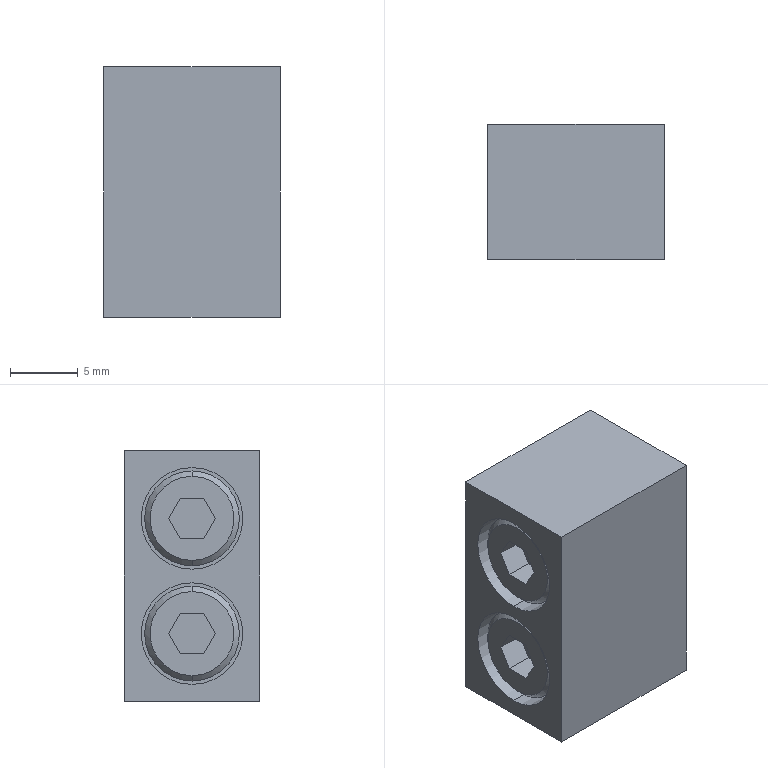Part | SolidWorks | features BaseBody 1 | 1 solid | 36 faces | box 13 x 10 x 18.5 mm | volume 2290 mm3 | plane 24 | cylinder 8 | cone 4 | commonest cylinder face diameters 7 x4 7.5 x4
STEP:
#1=CARTESIAN_POINT('',(-12.6,0.,7.35));
#2=VERTEX_POINT('',#1);
#3=CARTESIAN_POINT('',(-12.6,0.,1.15));
#4=VERTEX_POINT('',#3);
#5=CARTESIAN_POINT('',(-12.6,0.,4.25));
#6=DIRECTION('',(-1.,0.,0.));
#7=DIRECTION('',(0.,0.,1.));
#8=AXIS2_PLACEMENT_3D('',#5,#6,#7);
#9=CIRCLE('',#8,3.1);
#10=EDGE_CURVE('',#2,#4,#9,.T.);
#11=ORIENTED_EDGE('',*,*,#10,.F.);
#12=CARTESIAN_POINT('',(-12.2,0.,7.75));
#13=VERTEX_POINT('',#12);
#14=CARTESIAN_POINT('',(-12.2,0.,7.75));
#15=DIRECTION('',(0.7071,0.,0.7071));
#16=VECTOR('',#15,1000.);
#17=LINE('',#14,#16);
#18=EDGE_CURVE('',#2,#13,#17,.T.);
#19=ORIENTED_EDGE('',*,*,#18,.T.);
#20=CARTESIAN_POINT('',(-12.2,0.,0.75));
#21=VERTEX_POINT('',#20);
#22=CARTESIAN_POINT('',(-12.2,0.,4.25));
#23=DIRECTION('',(-1.,0.,0.));
#24=DIRECTION('',(0.,0.,1.));
#25=AXIS2_PLACEMENT_3D('',#22,#23,#24);
#26=CIRCLE('',#25,3.5);
#27=EDGE_CURVE('',#13,#21,#26,.T.);
#28=ORIENTED_EDGE('',*,*,#27,.T.);
#29=CARTESIAN_POINT('',(-12.2,0.,0.75));
#30=DIRECTION('',(0.7071,0.,-0.7071));
#31=VECTOR('',#30,1000.);
#32=LINE('',#29,#31);
#33=EDGE_CURVE('',#4,#21,#32,.T.);
#34=ORIENTED_EDGE('',*,*,#33,.F.);
#35=EDGE_LOOP('',(#11,#19,#28,#34));
#36=FACE_OUTER_BOUND('',#35,.T.);
#37=CARTESIAN_POINT('',(-12.2,0.,4.25));
#38=DIRECTION('',(1.,0.,0.));
#39=DIRECTION('',(0.,0.,-1.));
#40=AXIS2_PLACEMENT_3D('',#37,#38,#39);
#41=CONICAL_SURFACE('',#40,3.5,0.7854);
#42=ADVANCED_FACE('',(#36),#41,.T.);
#43=CARTESIAN_POINT('',(-8.6,0.,7.75));
#44=VERTEX_POINT('',#43);
#45=CARTESIAN_POINT('',(-8.6,0.,0.75));
#46=VERTEX_POINT('',#45);
#47=CARTESIAN_POINT('',(-8.6,0.,4.25));
#48=DIRECTION('',(-1.,0.,0.));
#49=DIRECTION('',(0.,0.,-1.));
#50=AXIS2_PLACEMENT_3D('',#47,#48,#49);
#51=CIRCLE('',#50,3.5);
#52=EDGE_CURVE('',#44,#46,#51,.T.);
#53=ORIENTED_EDGE('',*,*,#52,.T.);
#54=CARTESIAN_POINT('',(-12.6,0.,0.75));
#55=DIRECTION('',(-1.,0.,0.));
#56=VECTOR('',#55,1000.);
#57=LINE('',#54,#56);
#58=EDGE_CURVE('',#46,#21,#57,.T.);
#59=ORIENTED_EDGE('',*,*,#58,.T.);
#60=ORIENTED_EDGE('',*,*,#27,.F.);
#61=CARTESIAN_POINT('',(-12.6,0.,7.75));
#62=DIRECTION('',(-1.,0.,0.));
#63=VECTOR('',#62,1000.);
#64=LINE('',#61,#63);
#65=EDGE_CURVE('',#44,#13,#64,.T.);
#66=ORIENTED_EDGE('',*,*,#65,.F.);
#67=EDGE_LOOP('',(#53,#59,#60,#66));
#68=FACE_OUTER_BOUND('',#67,.T.);
#69=CARTESIAN_POINT('',(-12.6,0.,4.25));
#70=DIRECTION('',(-1.,0.,0.));
#71=DIRECTION('',(0.,0.,1.));
#72=AXIS2_PLACEMENT_3D('',#69,#70,#71);
#73=CYLINDRICAL_SURFACE('',#72,3.5);
#74=ADVANCED_FACE('',(#68),#73,.T.);
#75=CARTESIAN_POINT('',(-8.6,0.,8.));
#76=VERTEX_POINT('',#75);
#77=CARTESIAN_POINT('',(-8.6,0.,0.5));
#78=VERTEX_POINT('',#77);
#79=CARTESIAN_POINT('',(-8.6,0.,4.25));
#80=DIRECTION('',(1.,0.,0.));
#81=DIRECTION('',(0.,0.,-1.));
#82=AXIS2_PLACEMENT_3D('',#79,#80,#81);
#83=CIRCLE('',#82,3.75);
#84=EDGE_CURVE('',#76,#78,#83,.T.);
#85=ORIENTED_EDGE('',*,*,#84,.T.);
#86=CARTESIAN_POINT('',(-13.,0.,0.5));
#87=VERTEX_POINT('',#86);
#88=CARTESIAN_POINT('',(-8.6,0.,0.5));
#89=DIRECTION('',(-1.,0.,0.));
#90=VECTOR('',#89,1000.);
#91=LINE('',#88,#90);
#92=EDGE_CURVE('',#78,#87,#91,.T.);
#93=ORIENTED_EDGE('',*,*,#92,.T.);
#94=CARTESIAN_POINT('',(-13.,0.,8.));
#95=VERTEX_POINT('',#94);
#96=CARTESIAN_POINT('',(-13.,0.,4.25));
#97=DIRECTION('',(1.,0.,0.));
#98=DIRECTION('',(0.,0.,-1.));
#99=AXIS2_PLACEMENT_3D('',#96,#97,#98);
#100=CIRCLE('',#99,3.75);
#101=EDGE_CURVE('',#95,#87,#100,.T.);
#102=ORIENTED_EDGE('',*,*,#101,.F.);
#103=CARTESIAN_POINT('',(-8.6,0.,8.));
#104=DIRECTION('',(-1.,0.,0.));
#105=VECTOR('',#104,1000.);
#106=LINE('',#103,#105);
#107=EDGE_CURVE('',#76,#95,#106,.T.);
#108=ORIENTED_EDGE('',*,*,#107,.F.);
#109=EDGE_LOOP('',(#85,#93,#102,#108));
#110=FACE_OUTER_BOUND('',#109,.T.);
#111=CARTESIAN_POINT('',(-8.6,0.,4.25));
#112=DIRECTION('',(-1.,0.,0.));
#113=DIRECTION('',(0.,0.,1.));
#114=AXIS2_PLACEMENT_3D('',#111,#112,#113);
#115=CYLINDRICAL_SURFACE('',#114,3.75);
#116=ADVANCED_FACE('',(#110),#115,.F.);
#117=CARTESIAN_POINT('',(-8.6,0.,-0.5));
#118=VERTEX_POINT('',#117);
#119=CARTESIAN_POINT('',(-8.6,0.,-8.));
#120=VERTEX_POINT('',#119);
#121=CARTESIAN_POINT('',(-8.6,0.,-4.25));
#122=DIRECTION('',(1.,0.,0.));
#123=DIRECTION('',(0.,0.,-1.));
#124=AXIS2_PLACEMENT_3D('',#121,#122,#123);
#125=CIRCLE('',#124,3.75);
#126=EDGE_CURVE('',#118,#120,#125,.T.);
#127=ORIENTED_EDGE('',*,*,#126,.T.);
#128=CARTESIAN_POINT('',(-13.,0.,-8.));
#129=VERTEX_POINT('',#128);
#130=CARTESIAN_POINT('',(-8.6,0.,-8.));
#131=DIRECTION('',(-1.,0.,0.));
#132=VECTOR('',#131,1000.);
#133=LINE('',#130,#132);
#134=EDGE_CURVE('',#120,#129,#133,.T.);
#135=ORIENTED_EDGE('',*,*,#134,.T.);
#136=CARTESIAN_POINT('',(-13.,0.,-0.5));
#137=VERTEX_POINT('',#136);
#138=CARTESIAN_POINT('',(-13.,0.,-4.25));
#139=DIRECTION('',(1.,0.,0.));
#140=DIRECTION('',(0.,0.,-1.));
#141=AXIS2_PLACEMENT_3D('',#138,#139,#140);
#142=CIRCLE('',#141,3.75);
#143=EDGE_CURVE('',#137,#129,#142,.T.);
#144=ORIENTED_EDGE('',*,*,#143,.F.);
#145=CARTESIAN_POINT('',(-8.6,0.,-0.5));
#146=DIRECTION('',(-1.,0.,0.));
#147=VECTOR('',#146,1000.);
#148=LINE('',#145,#147);
#149=EDGE_CURVE('',#118,#137,#148,.T.);
#150=ORIENTED_EDGE('',*,*,#149,.F.);
#151=EDGE_LOOP('',(#127,#135,#144,#150));
#152=FACE_OUTER_BOUND('',#151,.T.);
#153=CARTESIAN_POINT('',(-8.6,0.,-4.25));
#154=DIRECTION('',(-1.,0.,0.));
#155=DIRECTION('',(0.,0.,1.));
#156=AXIS2_PLACEMENT_3D('',#153,#154,#155);
#157=CYLINDRICAL_SURFACE('',#156,3.75);
#158=ADVANCED_FACE('',(#152),#157,.F.);
#159=CARTESIAN_POINT('',(-8.6,0.,-0.75));
#160=VERTEX_POINT('',#159);
#161=CARTESIAN_POINT('',(-8.6,0.,-7.75));
#162=VERTEX_POINT('',#161);
#163=CARTESIAN_POINT('',(-8.6,0.,-4.25));
#164=DIRECTION('',(-1.,0.,0.));
#165=DIRECTION('',(0.,0.,-1.));
#166=AXIS2_PLACEMENT_3D('',#163,#164,#165);
#167=CIRCLE('',#166,3.5);
#168=EDGE_CURVE('',#160,#162,#167,.T.);
#169=ORIENTED_EDGE('',*,*,#168,.T.);
#170=CARTESIAN_POINT('',(-12.2,0.,-7.75));
#171=VERTEX_POINT('',#170);
#172=CARTESIAN_POINT('',(-12.6,0.,-7.75));
#173=DIRECTION('',(-1.,0.,0.));
#174=VECTOR('',#173,1000.);
#175=LINE('',#172,#174);
#176=EDGE_CURVE('',#162,#171,#175,.T.);
#177=ORIENTED_EDGE('',*,*,#176,.T.);
#178=CARTESIAN_POINT('',(-12.2,0.,-0.75));
#179=VERTEX_POINT('',#178);
#180=CARTESIAN_POINT('',(-12.2,0.,-4.25));
#181=DIRECTION('',(-1.,0.,0.));
#182=DIRECTION('',(0.,0.,1.));
#183=AXIS2_PLACEMENT_3D('',#180,#181,#182);
#184=CIRCLE('',#183,3.5);
#185=EDGE_CURVE('',#179,#171,#184,.T.);
#186=ORIENTED_EDGE('',*,*,#185,.F.);
#187=CARTESIAN_POINT('',(-12.6,0.,-0.75));
#188=DIRECTION('',(-1.,0.,0.));
#189=VECTOR('',#188,1000.);
#190=LINE('',#187,#189);
#191=EDGE_CURVE('',#160,#179,#190,.T.);
#192=ORIENTED_EDGE('',*,*,#191,.F.);
#193=EDGE_LOOP('',(#169,#177,#186,#192));
#194=FACE_OUTER_BOUND('',#193,.T.);
#195=CARTESIAN_POINT('',(-12.6,0.,-4.25));
#196=DIRECTION('',(-1.,0.,0.));
#197=DIRECTION('',(0.,0.,1.));
#198=AXIS2_PLACEMENT_3D('',#195,#196,#197);
#199=CYLINDRICAL_SURFACE('',#198,3.5);
#200=ADVANCED_FACE('',(#194),#199,.T.);
#201=CARTESIAN_POINT('',(-12.6,0.,-1.15));
#202=VERTEX_POINT('',#201);
#203=CARTESIAN_POINT('',(-12.6,0.,-7.35));
#204=VERTEX_POINT('',#203);
#205=CARTESIAN_POINT('',(-12.6,0.,-4.25));
#206=DIRECTION('',(-1.,0.,0.));
#207=DIRECTION('',(0.,0.,1.));
#208=AXIS2_PLACEMENT_3D('',#205,#206,#207);
#209=CIRCLE('',#208,3.1);
#210=EDGE_CURVE('',#202,#204,#209,.T.);
#211=ORIENTED_EDGE('',*,*,#210,.F.);
#212=CARTESIAN_POINT('',(-12.2,0.,-0.75));
#213=DIRECTION('',(0.7071,0.,0.7071));
#214=VECTOR('',#213,1000.);
#215=LINE('',#212,#214);
#216=EDGE_CURVE('',#202,#179,#215,.T.);
#217=ORIENTED_EDGE('',*,*,#216,.T.);
#218=ORIENTED_EDGE('',*,*,#185,.T.);
#219=CARTESIAN_POINT('',(-12.2,0.,-7.75));
#220=DIRECTION('',(0.7071,0.,-0.7071));
#221=VECTOR('',#220,1000.);
#222=LINE('',#219,#221);
#223=EDGE_CURVE('',#204,#171,#222,.T.);
#224=ORIENTED_EDGE('',*,*,#223,.F.);
#225=EDGE_LOOP('',(#211,#217,#218,#224));
#226=FACE_OUTER_BOUND('',#225,.T.);
#227=CARTESIAN_POINT('',(-12.2,0.,-4.25));
#228=DIRECTION('',(1.,0.,0.));
#229=DIRECTION('',(0.,0.,-1.));
#230=AXIS2_PLACEMENT_3D('',#227,#228,#229);
#231=CONICAL_SURFACE('',#230,3.5,0.7854);
#232=ADVANCED_FACE('',(#226),#231,.T.);
#233=CARTESIAN_POINT('',(-12.6,1.732,-4.25));
#234=VERTEX_POINT('',#233);
#235=CARTESIAN_POINT('',(-12.6,0.866,-2.75));
#236=VERTEX_POINT('',#235);
#237=CARTESIAN_POINT('',(-12.6,1.732,-4.25));
#238=DIRECTION('',(0.,-0.5,0.866));
#239=VECTOR('',#238,1000.);
#240=LINE('',#237,#239);
#241=EDGE_CURVE('',#234,#236,#240,.T.);
#242=ORIENTED_EDGE('',*,*,#241,.T.);
#243=CARTESIAN_POINT('',(-12.6,-0.866,-2.75));
#244=VERTEX_POINT('',#243);
#245=CARTESIAN_POINT('',(-12.6,-0.866,-2.75));
#246=DIRECTION('',(0.,1.,0.));
#247=VECTOR('',#246,1000.);
#248=LINE('',#245,#247);
#249=EDGE_CURVE('',#244,#236,#248,.T.);
#250=ORIENTED_EDGE('',*,*,#249,.F.);
#251=CARTESIAN_POINT('',(-12.6,-1.732,-4.25));
#252=VERTEX_POINT('',#251);
#253=CARTESIAN_POINT('',(-12.6,-0.866,-2.75));
#254=DIRECTION('',(0.,-0.5,-0.866));
#255=VECTOR('',#254,1000.);
#256=LINE('',#253,#255);
#257=EDGE_CURVE('',#244,#252,#256,.T.);
#258=ORIENTED_EDGE('',*,*,#257,.T.);
#259=CARTESIAN_POINT('',(-12.6,-0.866,-5.75));
#260=VERTEX_POINT('',#259);
#261=CARTESIAN_POINT('',(-12.6,-1.732,-4.25));
#262=DIRECTION('',(0.,0.5,-0.866));
#263=VECTOR('',#262,1000.);
#264=LINE('',#261,#263);
#265=EDGE_CURVE('',#252,#260,#264,.T.);
#266=ORIENTED_EDGE('',*,*,#265,.T.);
#267=CARTESIAN_POINT('',(-12.6,0.866,-5.75));
#268=VERTEX_POINT('',#267);
#269=CARTESIAN_POINT('',(-12.6,-0.866,-5.75));
#270=DIRECTION('',(0.,1.,0.));
#271=VECTOR('',#270,1000.);
#272=LINE('',#269,#271);
#273=EDGE_CURVE('',#260,#268,#272,.T.);
#274=ORIENTED_EDGE('',*,*,#273,.T.);
#275=CARTESIAN_POINT('',(-12.6,0.866,-5.75));
#276=DIRECTION('',(0.,0.5,0.866));
#277=VECTOR('',#276,1000.);
#278=LINE('',#275,#277);
#279=EDGE_CURVE('',#268,#234,#278,.T.);
#280=ORIENTED_EDGE('',*,*,#279,.T.);
#281=EDGE_LOOP('',(#242,#250,#258,#266,#274,#280));
#282=FACE_BOUND('',#281,.T.);
#283=CARTESIAN_POINT('',(-12.6,0.,-4.25));
#284=DIRECTION('',(-1.,0.,0.));
#285=DIRECTION('',(0.,0.,1.));
#286=AXIS2_PLACEMENT_3D('',#283,#284,#285);
#287=CIRCLE('',#286,3.1);
#288=EDGE_CURVE('',#204,#202,#287,.T.);
#289=ORIENTED_EDGE('',*,*,#288,.T.);
#290=ORIENTED_EDGE('',*,*,#210,.T.);
#291=EDGE_LOOP('',(#289,#290));
#292=FACE_OUTER_BOUND('',#291,.T.);
#293=CARTESIAN_POINT('',(-12.6,0.,-1.15));
#294=DIRECTION('',(1.,0.,0.));
#295=DIRECTION('',(0.,0.,-1.));
#296=AXIS2_PLACEMENT_3D('',#293,#294,#295);
#297=PLANE('',#296);
#298=ADVANCED_FACE('',(#282,#292),#297,.F.);
#299=ORIENTED_EDGE('',*,*,#241,.F.);
#300=CARTESIAN_POINT('',(-10.6,1.732,-4.25));
#301=VERTEX_POINT('',#300);
#302=CARTESIAN_POINT('',(-10.6,1.732,-4.25));
#303=DIRECTION('',(-1.,0.,0.));
#304=VECTOR('',#303,1000.);
#305=LINE('',#302,#304);
#306=EDGE_CURVE('',#301,#234,#305,.T.);
#307=ORIENTED_EDGE('',*,*,#306,.F.);
#308=CARTESIAN_POINT('',(-10.6,0.866,-2.75));
#309=VERTEX_POINT('',#308);
#310=CARTESIAN_POINT('',(-10.6,1.732,-4.25));
#311=DIRECTION('',(0.,-0.5,0.866));
#312=VECTOR('',#311,1000.);
#313=LINE('',#310,#312);
#314=EDGE_CURVE('',#301,#309,#313,.T.);
#315=ORIENTED_EDGE('',*,*,#314,.T.);
#316=CARTESIAN_POINT('',(-10.6,0.866,-2.75));
#317=DIRECTION('',(-1.,0.,0.));
#318=VECTOR('',#317,1000.);
#319=LINE('',#316,#318);
#320=EDGE_CURVE('',#309,#236,#319,.T.);
#321=ORIENTED_EDGE('',*,*,#320,.T.);
#322=EDGE_LOOP('',(#299,#307,#315,#321));
#323=FACE_OUTER_BOUND('',#322,.T.);
#324=CARTESIAN_POINT('',(-10.6,1.732,-4.25));
#325=DIRECTION('',(0.,-0.866,-0.5));
#326=DIRECTION('',(0.,0.5,-0.866));
#327=AXIS2_PLACEMENT_3D('',#324,#325,#326);
#328=PLANE('',#327);
#329=ADVANCED_FACE('',(#323),#328,.T.);
#330=ORIENTED_EDGE('',*,*,#249,.T.);
#331=ORIENTED_EDGE('',*,*,#320,.F.);
#332=CARTESIAN_POINT('',(-10.6,-0.866,-2.75));
#333=VERTEX_POINT('',#332);
#334=CARTESIAN_POINT('',(-10.6,0.866,-2.75));
#335=DIRECTION('',(0.,-1.,0.));
#336=VECTOR('',#335,1000.);
#337=LINE('',#334,#336);
#338=EDGE_CURVE('',#309,#333,#337,.T.);
#339=ORIENTED_EDGE('',*,*,#338,.T.);
#340=CARTESIAN_POINT('',(-10.6,-0.866,-2.75));
#341=DIRECTION('',(-1.,0.,0.));
#342=VECTOR('',#341,1000.);
#343=LINE('',#340,#342);
#344=EDGE_CURVE('',#333,#244,#343,.T.);
#345=ORIENTED_EDGE('',*,*,#344,.T.);
#346=EDGE_LOOP('',(#330,#331,#339,#345));
#347=FACE_OUTER_BOUND('',#346,.T.);
#348=CARTESIAN_POINT('',(-10.6,0.866,-2.75));
#349=DIRECTION('',(0.,0.,-1.));
#350=DIRECTION('',(-1.,0.,0.));
#351=AXIS2_PLACEMENT_3D('',#348,#349,#350);
#352=PLANE('',#351);
#353=ADVANCED_FACE('',(#347),#352,.T.);
#354=ORIENTED_EDGE('',*,*,#257,.F.);
#355=ORIENTED_EDGE('',*,*,#344,.F.);
#356=CARTESIAN_POINT('',(-10.6,-1.732,-4.25));
#357=VERTEX_POINT('',#356);
#358=CARTESIAN_POINT('',(-10.6,-0.866,-2.75));
#359=DIRECTION('',(0.,-0.5,-0.866));
#360=VECTOR('',#359,1000.);
#361=LINE('',#358,#360);
#362=EDGE_CURVE('',#333,#357,#361,.T.);
#363=ORIENTED_EDGE('',*,*,#362,.T.);
#364=CARTESIAN_POINT('',(-10.6,-1.732,-4.25));
#365=DIRECTION('',(-1.,0.,0.));
#366=VECTOR('',#365,1000.);
#367=LINE('',#364,#366);
#368=EDGE_CURVE('',#357,#252,#367,.T.);
#369=ORIENTED_EDGE('',*,*,#368,.T.);
#370=EDGE_LOOP('',(#354,#355,#363,#369));
#371=FACE_OUTER_BOUND('',#370,.T.);
#372=CARTESIAN_POINT('',(-10.6,-0.866,-2.75));
#373=DIRECTION('',(0.,0.866,-0.5));
#374=DIRECTION('',(0.,0.5,0.866));
#375=AXIS2_PLACEMENT_3D('',#372,#373,#374);
#376=PLANE('',#375);
#377=ADVANCED_FACE('',(#371),#376,.T.);
#378=ORIENTED_EDGE('',*,*,#265,.F.);
#379=ORIENTED_EDGE('',*,*,#368,.F.);
#380=CARTESIAN_POINT('',(-10.6,-0.866,-5.75));
#381=VERTEX_POINT('',#380);
#382=CARTESIAN_POINT('',(-10.6,-1.732,-4.25));
#383=DIRECTION('',(0.,0.5,-0.866));
#384=VECTOR('',#383,1000.);
#385=LINE('',#382,#384);
#386=EDGE_CURVE('',#357,#381,#385,.T.);
#387=ORIENTED_EDGE('',*,*,#386,.T.);
#388=CARTESIAN_POINT('',(-10.6,-0.866,-5.75));
#389=DIRECTION('',(-1.,0.,0.));
#390=VECTOR('',#389,1000.);
#391=LINE('',#388,#390);
#392=EDGE_CURVE('',#381,#260,#391,.T.);
#393=ORIENTED_EDGE('',*,*,#392,.T.);
#394=EDGE_LOOP('',(#378,#379,#387,#393));
#395=FACE_OUTER_BOUND('',#394,.T.);
#396=CARTESIAN_POINT('',(-10.6,-1.732,-4.25));
#397=DIRECTION('',(0.,0.866,0.5));
#398=DIRECTION('',(0.,-0.5,0.866));
#399=AXIS2_PLACEMENT_3D('',#396,#397,#398);
#400=PLANE('',#399);
#401=ADVANCED_FACE('',(#395),#400,.T.);
#402=ORIENTED_EDGE('',*,*,#273,.F.);
#403=ORIENTED_EDGE('',*,*,#392,.F.);
#404=CARTESIAN_POINT('',(-10.6,0.866,-5.75));
#405=VERTEX_POINT('',#404);
#406=CARTESIAN_POINT('',(-10.6,-0.866,-5.75));
#407=DIRECTION('',(0.,1.,0.));
#408=VECTOR('',#407,1000.);
#409=LINE('',#406,#408);
#410=EDGE_CURVE('',#381,#405,#409,.T.);
#411=ORIENTED_EDGE('',*,*,#410,.T.);
#412=CARTESIAN_POINT('',(-10.6,0.866,-5.75));
#413=DIRECTION('',(-1.,0.,0.));
#414=VECTOR('',#413,1000.);
#415=LINE('',#412,#414);
#416=EDGE_CURVE('',#405,#268,#415,.T.);
#417=ORIENTED_EDGE('',*,*,#416,.T.);
#418=EDGE_LOOP('',(#402,#403,#411,#417));
#419=FACE_OUTER_BOUND('',#418,.T.);
#420=CARTESIAN_POINT('',(-10.6,-0.866,-5.75));
#421=DIRECTION('',(0.,0.,1.));
#422=DIRECTION('',(1.,0.,0.));
#423=AXIS2_PLACEMENT_3D('',#420,#421,#422);
#424=PLANE('',#423);
#425=ADVANCED_FACE('',(#419),#424,.T.);
#426=ORIENTED_EDGE('',*,*,#279,.F.);
#427=ORIENTED_EDGE('',*,*,#416,.F.);
#428=CARTESIAN_POINT('',(-10.6,0.866,-5.75));
#429=DIRECTION('',(0.,0.5,0.866));
#430=VECTOR('',#429,1000.);
#431=LINE('',#428,#430);
#432=EDGE_CURVE('',#405,#301,#431,.T.);
#433=ORIENTED_EDGE('',*,*,#432,.T.);
#434=ORIENTED_EDGE('',*,*,#306,.T.);
#435=EDGE_LOOP('',(#426,#427,#433,#434));
#436=FACE_OUTER_BOUND('',#435,.T.);
#437=CARTESIAN_POINT('',(-10.6,0.866,-5.75));
#438=DIRECTION('',(0.,-0.866,0.5));
#439=DIRECTION('',(0.,-0.5,-0.866));
#440=AXIS2_PLACEMENT_3D('',#437,#438,#439);
#441=PLANE('',#440);
#442=ADVANCED_FACE('',(#436),#441,.T.);
#443=ORIENTED_EDGE('',*,*,#216,.F.);
#444=ORIENTED_EDGE('',*,*,#288,.F.);
#445=ORIENTED_EDGE('',*,*,#223,.T.);
#446=CARTESIAN_POINT('',(-12.2,0.,-4.25));
#447=DIRECTION('',(-1.,0.,0.));
#448=DIRECTION('',(0.,0.,1.));
#449=AXIS2_PLACEMENT_3D('',#446,#447,#448);
#450=CIRCLE('',#449,3.5);
#451=EDGE_CURVE('',#171,#179,#450,.T.);
#452=ORIENTED_EDGE('',*,*,#451,.T.);
#453=EDGE_LOOP('',(#443,#444,#445,#452));
#454=FACE_OUTER_BOUND('',#453,.T.);
#455=CARTESIAN_POINT('',(-12.2,0.,-4.25));
#456=DIRECTION('',(1.,0.,0.));
#457=DIRECTION('',(0.,0.,-1.));
#458=AXIS2_PLACEMENT_3D('',#455,#456,#457);
#459=CONICAL_SURFACE('',#458,3.5,0.7854);
#460=ADVANCED_FACE('',(#454),#459,.T.);
#461=ORIENTED_EDGE('',*,*,#338,.F.);
#462=ORIENTED_EDGE('',*,*,#314,.F.);
#463=ORIENTED_EDGE('',*,*,#432,.F.);
#464=ORIENTED_EDGE('',*,*,#410,.F.);
#465=ORIENTED_EDGE('',*,*,#386,.F.);
#466=ORIENTED_EDGE('',*,*,#362,.F.);
#467=EDGE_LOOP('',(#461,#462,#463,#464,#465,#466));
#468=FACE_OUTER_BOUND('',#467,.T.);
#469=CARTESIAN_POINT('',(-10.6,0.,-8.5));
#470=DIRECTION('',(1.,0.,0.));
#471=DIRECTION('',(0.,0.,-1.));
#472=AXIS2_PLACEMENT_3D('',#469,#470,#471);
#473=PLANE('',#472);
#474=ADVANCED_FACE('',(#468),#473,.F.);
#475=ORIENTED_EDGE('',*,*,#176,.F.);
#476=CARTESIAN_POINT('',(-8.6,0.,-4.25));
#477=DIRECTION('',(-1.,0.,0.));
#478=DIRECTION('',(0.,0.,-1.));
#479=AXIS2_PLACEMENT_3D('',#476,#477,#478);
#480=CIRCLE('',#479,3.5);
#481=EDGE_CURVE('',#162,#160,#480,.T.);
#482=ORIENTED_EDGE('',*,*,#481,.T.);
#483=ORIENTED_EDGE('',*,*,#191,.T.);
#484=ORIENTED_EDGE('',*,*,#451,.F.);
#485=EDGE_LOOP('',(#475,#482,#483,#484));
#486=FACE_OUTER_BOUND('',#485,.T.);
#487=CARTESIAN_POINT('',(-12.6,0.,-4.25));
#488=DIRECTION('',(-1.,0.,0.));
#489=DIRECTION('',(0.,0.,1.));
#490=AXIS2_PLACEMENT_3D('',#487,#488,#489);
#491=CYLINDRICAL_SURFACE('',#490,3.5);
#492=ADVANCED_FACE('',(#486),#491,.T.);
#493=ORIENTED_EDGE('',*,*,#168,.F.);
#494=ORIENTED_EDGE('',*,*,#481,.F.);
#495=EDGE_LOOP('',(#493,#494));
#496=FACE_BOUND('',#495,.T.);
#497=ORIENTED_EDGE('',*,*,#126,.F.);
#498=CARTESIAN_POINT('',(-8.6,0.,-4.25));
#499=DIRECTION('',(1.,0.,0.));
#500=DIRECTION('',(0.,0.,-1.));
#501=AXIS2_PLACEMENT_3D('',#498,#499,#500);
#502=CIRCLE('',#501,3.75);
#503=EDGE_CURVE('',#120,#118,#502,.T.);
#504=ORIENTED_EDGE('',*,*,#503,.F.);
#505=EDGE_LOOP('',(#497,#504));
#506=FACE_OUTER_BOUND('',#505,.T.);
#507=CARTESIAN_POINT('',(-8.6,0.,-4.25));
#508=DIRECTION('',(1.,0.,0.));
#509=DIRECTION('',(0.,0.,-1.));
#510=AXIS2_PLACEMENT_3D('',#507,#508,#509);
#511=PLANE('',#510);
#512=ADVANCED_FACE('',(#496,#506),#511,.F.);
#513=ORIENTED_EDGE('',*,*,#134,.F.);
#514=ORIENTED_EDGE('',*,*,#503,.T.);
#515=ORIENTED_EDGE('',*,*,#149,.T.);
#516=CARTESIAN_POINT('',(-13.,0.,-4.25));
#517=DIRECTION('',(1.,0.,0.));
#518=DIRECTION('',(0.,0.,-1.));
#519=AXIS2_PLACEMENT_3D('',#516,#517,#518);
#520=CIRCLE('',#519,3.75);
#521=EDGE_CURVE('',#129,#137,#520,.T.);
#522=ORIENTED_EDGE('',*,*,#521,.F.);
#523=EDGE_LOOP('',(#513,#514,#515,#522));
#524=FACE_OUTER_BOUND('',#523,.T.);
#525=CARTESIAN_POINT('',(-8.6,0.,-4.25));
#526=DIRECTION('',(-1.,0.,0.));
#527=DIRECTION('',(0.,0.,1.));
#528=AXIS2_PLACEMENT_3D('',#525,#526,#527);
#529=CYLINDRICAL_SURFACE('',#528,3.75);
#530=ADVANCED_FACE('',(#524),#529,.F.);
#531=ORIENTED_EDGE('',*,*,#143,.T.);
#532=ORIENTED_EDGE('',*,*,#521,.T.);
#533=EDGE_LOOP('',(#531,#532));
#534=FACE_BOUND('',#533,.T.);
#535=ORIENTED_EDGE('',*,*,#101,.T.);
#536=CARTESIAN_POINT('',(-13.,0.,4.25));
#537=DIRECTION('',(1.,0.,0.));
#538=DIRECTION('',(0.,0.,-1.));
#539=AXIS2_PLACEMENT_3D('',#536,#537,#538);
#540=CIRCLE('',#539,3.75);
#541=EDGE_CURVE('',#87,#95,#540,.T.);
#542=ORIENTED_EDGE('',*,*,#541,.T.);
#543=EDGE_LOOP('',(#535,#542));
#544=FACE_BOUND('',#543,.T.);
#545=CARTESIAN_POINT('',(-13.,-5.,-9.25));
#546=VERTEX_POINT('',#545);
#547=CARTESIAN_POINT('',(-13.,-5.,9.25));
#548=VERTEX_POINT('',#547);
#549=CARTESIAN_POINT('',(-13.,-5.,-9.25));
#550=DIRECTION('',(0.,0.,1.));
#551=VECTOR('',#550,1000.);
#552=LINE('',#549,#551);
#553=EDGE_CURVE('',#546,#548,#552,.T.);
#554=ORIENTED_EDGE('',*,*,#553,.T.);
#555=CARTESIAN_POINT('',(-13.,5.,9.25));
#556=VERTEX_POINT('',#555);
#557=CARTESIAN_POINT('',(-13.,5.,9.25));
#558=DIRECTION('',(0.,-1.,0.));
#559=VECTOR('',#558,1000.);
#560=LINE('',#557,#559);
#561=EDGE_CURVE('',#556,#548,#560,.T.);
#562=ORIENTED_EDGE('',*,*,#561,.F.);
#563=CARTESIAN_POINT('',(-13.,5.,-9.25));
#564=VERTEX_POINT('',#563);
#565=CARTESIAN_POINT('',(-13.,5.,-9.25));
#566=DIRECTION('',(0.,0.,1.));
#567=VECTOR('',#566,1000.);
#568=LINE('',#565,#567);
#569=EDGE_CURVE('',#564,#556,#568,.T.);
#570=ORIENTED_EDGE('',*,*,#569,.F.);
#571=CARTESIAN_POINT('',(-13.,5.,-9.25));
#572=DIRECTION('',(0.,-1.,0.));
#573=VECTOR('',#572,1000.);
#574=LINE('',#571,#573);
#575=EDGE_CURVE('',#564,#546,#574,.T.);
#576=ORIENTED_EDGE('',*,*,#575,.T.);
#577=EDGE_LOOP('',(#554,#562,#570,#576));
#578=FACE_OUTER_BOUND('',#577,.T.);
#579=CARTESIAN_POINT('',(-13.,5.,-9.25));
#580=DIRECTION('',(1.,0.,0.));
#581=DIRECTION('',(0.,0.,-1.));
#582=AXIS2_PLACEMENT_3D('',#579,#580,#581);
#583=PLANE('',#582);
#584=ADVANCED_FACE('',(#534,#544,#578),#583,.F.);
#585=ORIENTED_EDGE('',*,*,#92,.F.);
#586=CARTESIAN_POINT('',(-8.6,0.,4.25));
#587=DIRECTION('',(1.,0.,0.));
#588=DIRECTION('',(0.,0.,-1.));
#589=AXIS2_PLACEMENT_3D('',#586,#587,#588);
#590=CIRCLE('',#589,3.75);
#591=EDGE_CURVE('',#78,#76,#590,.T.);
#592=ORIENTED_EDGE('',*,*,#591,.T.);
#593=ORIENTED_EDGE('',*,*,#107,.T.);
#594=ORIENTED_EDGE('',*,*,#541,.F.);
#595=EDGE_LOOP('',(#585,#592,#593,#594));
#596=FACE_OUTER_BOUND('',#595,.T.);
#597=CARTESIAN_POINT('',(-8.6,0.,4.25));
#598=DIRECTION('',(-1.,0.,0.));
#599=DIRECTION('',(0.,0.,1.));
#600=AXIS2_PLACEMENT_3D('',#597,#598,#599);
#601=CYLINDRICAL_SURFACE('',#600,3.75);
#602=ADVANCED_FACE('',(#596),#601,.F.);
#603=CARTESIAN_POINT('',(0.,-5.,-9.25));
#604=VERTEX_POINT('',#603);
#605=CARTESIAN_POINT('',(0.,-5.,-9.25));
#606=DIRECTION('',(-1.,0.,0.));
#607=VECTOR('',#606,1000.);
#608=LINE('',#605,#607);
#609=EDGE_CURVE('',#604,#546,#608,.T.);
#610=ORIENTED_EDGE('',*,*,#609,.F.);
#611=CARTESIAN_POINT('',(0.,-5.,9.25));
#612=VERTEX_POINT('',#611);
#613=CARTESIAN_POINT('',(0.,-5.,9.25));
#614=DIRECTION('',(0.,0.,-1.));
#615=VECTOR('',#614,1000.);
#616=LINE('',#613,#615);
#617=EDGE_CURVE('',#612,#604,#616,.T.);
#618=ORIENTED_EDGE('',*,*,#617,.F.);
#619=CARTESIAN_POINT('',(-13.,-5.,9.25));
#620=DIRECTION('',(1.,0.,0.));
#621=VECTOR('',#620,1000.);
#622=LINE('',#619,#621);
#623=EDGE_CURVE('',#548,#612,#622,.T.);
#624=ORIENTED_EDGE('',*,*,#623,.F.);
#625=ORIENTED_EDGE('',*,*,#553,.F.);
#626=EDGE_LOOP('',(#610,#618,#624,#625));
#627=FACE_OUTER_BOUND('',#626,.T.);
#628=CARTESIAN_POINT('',(0.,-5.,0.));
#629=DIRECTION('',(0.,1.,0.));
#630=DIRECTION('',(0.,0.,1.));
#631=AXIS2_PLACEMENT_3D('',#628,#629,#630);
#632=PLANE('',#631);
#633=ADVANCED_FACE('',(#627),#632,.F.);
#634=ORIENTED_EDGE('',*,*,#623,.T.);
#635=CARTESIAN_POINT('',(0.,5.,9.25));
#636=VERTEX_POINT('',#635);
#637=CARTESIAN_POINT('',(0.,5.,9.25));
#638=DIRECTION('',(0.,-1.,0.));
#639=VECTOR('',#638,1000.);
#640=LINE('',#637,#639);
#641=EDGE_CURVE('',#636,#612,#640,.T.);
#642=ORIENTED_EDGE('',*,*,#641,.F.);
#643=CARTESIAN_POINT('',(-13.,5.,9.25));
#644=DIRECTION('',(1.,0.,0.));
#645=VECTOR('',#644,1000.);
#646=LINE('',#643,#645);
#647=EDGE_CURVE('',#556,#636,#646,.T.);
#648=ORIENTED_EDGE('',*,*,#647,.F.);
#649=ORIENTED_EDGE('',*,*,#561,.T.);
#650=EDGE_LOOP('',(#634,#642,#648,#649));
#651=FACE_OUTER_BOUND('',#650,.T.);
#652=CARTESIAN_POINT('',(-13.,5.,9.25));
#653=DIRECTION('',(0.,0.,-1.));
#654=DIRECTION('',(-1.,0.,0.));
#655=AXIS2_PLACEMENT_3D('',#652,#653,#654);
#656=PLANE('',#655);
#657=ADVANCED_FACE('',(#651),#656,.F.);
#658=CARTESIAN_POINT('',(0.,5.,-9.25));
#659=VERTEX_POINT('',#658);
#660=CARTESIAN_POINT('',(0.,5.,-9.25));
#661=DIRECTION('',(-1.,0.,0.));
#662=VECTOR('',#661,1000.);
#663=LINE('',#660,#662);
#664=EDGE_CURVE('',#659,#564,#663,.T.);
#665=ORIENTED_EDGE('',*,*,#664,.T.);
#666=ORIENTED_EDGE('',*,*,#569,.T.);
#667=ORIENTED_EDGE('',*,*,#647,.T.);
#668=CARTESIAN_POINT('',(0.,5.,9.25));
#669=DIRECTION('',(0.,0.,-1.));
#670=VECTOR('',#669,1000.);
#671=LINE('',#668,#670);
#672=EDGE_CURVE('',#636,#659,#671,.T.);
#673=ORIENTED_EDGE('',*,*,#672,.T.);
#674=EDGE_LOOP('',(#665,#666,#667,#673));
#675=FACE_OUTER_BOUND('',#674,.T.);
#676=CARTESIAN_POINT('',(0.,5.,0.));
#677=DIRECTION('',(0.,1.,0.));
#678=DIRECTION('',(0.,0.,1.));
#679=AXIS2_PLACEMENT_3D('',#676,#677,#678);
#680=PLANE('',#679);
#681=ADVANCED_FACE('',(#675),#680,.T.);
#682=ORIENTED_EDGE('',*,*,#609,.T.);
#683=ORIENTED_EDGE('',*,*,#575,.F.);
#684=ORIENTED_EDGE('',*,*,#664,.F.);
#685=CARTESIAN_POINT('',(0.,5.,-9.25));
#686=DIRECTION('',(0.,-1.,0.));
#687=VECTOR('',#686,1000.);
#688=LINE('',#685,#687);
#689=EDGE_CURVE('',#659,#604,#688,.T.);
#690=ORIENTED_EDGE('',*,*,#689,.T.);
#691=EDGE_LOOP('',(#682,#683,#684,#690));
#692=FACE_OUTER_BOUND('',#691,.T.);
#693=CARTESIAN_POINT('',(0.,5.,-9.25));
#694=DIRECTION('',(0.,0.,1.));
#695=DIRECTION('',(1.,0.,0.));
#696=AXIS2_PLACEMENT_3D('',#693,#694,#695);
#697=PLANE('',#696);
#698=ADVANCED_FACE('',(#692),#697,.F.);
#699=ORIENTED_EDGE('',*,*,#52,.F.);
#700=CARTESIAN_POINT('',(-8.6,0.,4.25));
#701=DIRECTION('',(-1.,0.,0.));
#702=DIRECTION('',(0.,0.,-1.));
#703=AXIS2_PLACEMENT_3D('',#700,#701,#702);
#704=CIRCLE('',#703,3.5);
#705=EDGE_CURVE('',#46,#44,#704,.T.);
#706=ORIENTED_EDGE('',*,*,#705,.F.);
#707=EDGE_LOOP('',(#699,#706));
#708=FACE_BOUND('',#707,.T.);
#709=ORIENTED_EDGE('',*,*,#84,.F.);
#710=ORIENTED_EDGE('',*,*,#591,.F.);
#711=EDGE_LOOP('',(#709,#710));
#712=FACE_OUTER_BOUND('',#711,.T.);
#713=CARTESIAN_POINT('',(-8.6,0.,4.25));
#714=DIRECTION('',(1.,0.,0.));
#715=DIRECTION('',(0.,0.,-1.));
#716=AXIS2_PLACEMENT_3D('',#713,#714,#715);
#717=PLANE('',#716);
#718=ADVANCED_FACE('',(#708,#712),#717,.F.);
#719=ORIENTED_EDGE('',*,*,#617,.T.);
#720=ORIENTED_EDGE('',*,*,#689,.F.);
#721=ORIENTED_EDGE('',*,*,#672,.F.);
#722=ORIENTED_EDGE('',*,*,#641,.T.);
#723=EDGE_LOOP('',(#719,#720,#721,#722));
#724=FACE_OUTER_BOUND('',#723,.T.);
#725=CARTESIAN_POINT('',(0.,5.,9.25));
#726=DIRECTION('',(-1.,0.,0.));
#727=DIRECTION('',(0.,0.,1.));
#728=AXIS2_PLACEMENT_3D('',#725,#726,#727);
#729=PLANE('',#728);
#730=ADVANCED_FACE('',(#724),#729,.F.);
#731=ORIENTED_EDGE('',*,*,#58,.F.);
#732=ORIENTED_EDGE('',*,*,#705,.T.);
#733=ORIENTED_EDGE('',*,*,#65,.T.);
#734=CARTESIAN_POINT('',(-12.2,0.,4.25));
#735=DIRECTION('',(-1.,0.,0.));
#736=DIRECTION('',(0.,0.,1.));
#737=AXIS2_PLACEMENT_3D('',#734,#735,#736);
#738=CIRCLE('',#737,3.5);
#739=EDGE_CURVE('',#21,#13,#738,.T.);
#740=ORIENTED_EDGE('',*,*,#739,.F.);
#741=EDGE_LOOP('',(#731,#732,#733,#740));
#742=FACE_OUTER_BOUND('',#741,.T.);
#743=CARTESIAN_POINT('',(-12.6,0.,4.25));
#744=DIRECTION('',(-1.,0.,0.));
#745=DIRECTION('',(0.,0.,1.));
#746=AXIS2_PLACEMENT_3D('',#743,#744,#745);
#747=CYLINDRICAL_SURFACE('',#746,3.5);
#748=ADVANCED_FACE('',(#742),#747,.T.);
#749=ORIENTED_EDGE('',*,*,#18,.F.);
#750=CARTESIAN_POINT('',(-12.6,0.,4.25));
#751=DIRECTION('',(-1.,0.,0.));
#752=DIRECTION('',(0.,0.,1.));
#753=AXIS2_PLACEMENT_3D('',#750,#751,#752);
#754=CIRCLE('',#753,3.1);
#755=EDGE_CURVE('',#4,#2,#754,.T.);
#756=ORIENTED_EDGE('',*,*,#755,.F.);
#757=ORIENTED_EDGE('',*,*,#33,.T.);
#758=ORIENTED_EDGE('',*,*,#739,.T.);
#759=EDGE_LOOP('',(#749,#756,#757,#758));
#760=FACE_OUTER_BOUND('',#759,.T.);
#761=CARTESIAN_POINT('',(-12.2,0.,4.25));
#762=DIRECTION('',(1.,0.,0.));
#763=DIRECTION('',(0.,0.,-1.));
#764=AXIS2_PLACEMENT_3D('',#761,#762,#763);
#765=CONICAL_SURFACE('',#764,3.5,0.7854);
#766=ADVANCED_FACE('',(#760),#765,.T.);
#767=CARTESIAN_POINT('',(-12.6,1.732,4.25));
#768=VERTEX_POINT('',#767);
#769=CARTESIAN_POINT('',(-12.6,0.866,5.75));
#770=VERTEX_POINT('',#769);
#771=CARTESIAN_POINT('',(-12.6,1.732,4.25));
#772=DIRECTION('',(0.,-0.5,0.866));
#773=VECTOR('',#772,1000.);
#774=LINE('',#771,#773);
#775=EDGE_CURVE('',#768,#770,#774,.T.);
#776=ORIENTED_EDGE('',*,*,#775,.T.);
#777=CARTESIAN_POINT('',(-12.6,-0.866,5.75));
#778=VERTEX_POINT('',#777);
#779=CARTESIAN_POINT('',(-12.6,-0.866,5.75));
#780=DIRECTION('',(0.,1.,0.));
#781=VECTOR('',#780,1000.);
#782=LINE('',#779,#781);
#783=EDGE_CURVE('',#778,#770,#782,.T.);
#784=ORIENTED_EDGE('',*,*,#783,.F.);
#785=CARTESIAN_POINT('',(-12.6,-1.732,4.25));
#786=VERTEX_POINT('',#785);
#787=CARTESIAN_POINT('',(-12.6,-0.866,5.75));
#788=DIRECTION('',(0.,-0.5,-0.866));
#789=VECTOR('',#788,1000.);
#790=LINE('',#787,#789);
#791=EDGE_CURVE('',#778,#786,#790,.T.);
#792=ORIENTED_EDGE('',*,*,#791,.T.);
#793=CARTESIAN_POINT('',(-12.6,-0.866,2.75));
#794=VERTEX_POINT('',#793);
#795=CARTESIAN_POINT('',(-12.6,-1.732,4.25));
#796=DIRECTION('',(0.,0.5,-0.866));
#797=VECTOR('',#796,1000.);
#798=LINE('',#795,#797);
#799=EDGE_CURVE('',#786,#794,#798,.T.);
#800=ORIENTED_EDGE('',*,*,#799,.T.);
#801=CARTESIAN_POINT('',(-12.6,0.866,2.75));
#802=VERTEX_POINT('',#801);
#803=CARTESIAN_POINT('',(-12.6,-0.866,2.75));
#804=DIRECTION('',(0.,1.,0.));
#805=VECTOR('',#804,1000.);
#806=LINE('',#803,#805);
#807=EDGE_CURVE('',#794,#802,#806,.T.);
#808=ORIENTED_EDGE('',*,*,#807,.T.);
#809=CARTESIAN_POINT('',(-12.6,0.866,2.75));
#810=DIRECTION('',(0.,0.5,0.866));
#811=VECTOR('',#810,1000.);
#812=LINE('',#809,#811);
#813=EDGE_CURVE('',#802,#768,#812,.T.);
#814=ORIENTED_EDGE('',*,*,#813,.T.);
#815=EDGE_LOOP('',(#776,#784,#792,#800,#808,#814));
#816=FACE_BOUND('',#815,.T.);
#817=ORIENTED_EDGE('',*,*,#755,.T.);
#818=ORIENTED_EDGE('',*,*,#10,.T.);
#819=EDGE_LOOP('',(#817,#818));
#820=FACE_OUTER_BOUND('',#819,.T.);
#821=CARTESIAN_POINT('',(-12.6,0.,7.35));
#822=DIRECTION('',(1.,0.,0.));
#823=DIRECTION('',(0.,0.,-1.));
#824=AXIS2_PLACEMENT_3D('',#821,#822,#823);
#825=PLANE('',#824);
#826=ADVANCED_FACE('',(#816,#820),#825,.F.);
#827=ORIENTED_EDGE('',*,*,#775,.F.);
#828=CARTESIAN_POINT('',(-10.6,1.732,4.25));
#829=VERTEX_POINT('',#828);
#830=CARTESIAN_POINT('',(-10.6,1.732,4.25));
#831=DIRECTION('',(-1.,0.,0.));
#832=VECTOR('',#831,1000.);
#833=LINE('',#830,#832);
#834=EDGE_CURVE('',#829,#768,#833,.T.);
#835=ORIENTED_EDGE('',*,*,#834,.F.);
#836=CARTESIAN_POINT('',(-10.6,0.866,5.75));
#837=VERTEX_POINT('',#836);
#838=CARTESIAN_POINT('',(-10.6,1.732,4.25));
#839=DIRECTION('',(0.,-0.5,0.866));
#840=VECTOR('',#839,1000.);
#841=LINE('',#838,#840);
#842=EDGE_CURVE('',#829,#837,#841,.T.);
#843=ORIENTED_EDGE('',*,*,#842,.T.);
#844=CARTESIAN_POINT('',(-10.6,0.866,5.75));
#845=DIRECTION('',(-1.,0.,0.));
#846=VECTOR('',#845,1000.);
#847=LINE('',#844,#846);
#848=EDGE_CURVE('',#837,#770,#847,.T.);
#849=ORIENTED_EDGE('',*,*,#848,.T.);
#850=EDGE_LOOP('',(#827,#835,#843,#849));
#851=FACE_OUTER_BOUND('',#850,.T.);
#852=CARTESIAN_POINT('',(-10.6,1.732,4.25));
#853=DIRECTION('',(0.,-0.866,-0.5));
#854=DIRECTION('',(0.,0.5,-0.866));
#855=AXIS2_PLACEMENT_3D('',#852,#853,#854);
#856=PLANE('',#855);
#857=ADVANCED_FACE('',(#851),#856,.T.);
#858=ORIENTED_EDGE('',*,*,#783,.T.);
#859=ORIENTED_EDGE('',*,*,#848,.F.);
#860=CARTESIAN_POINT('',(-10.6,-0.866,5.75));
#861=VERTEX_POINT('',#860);
#862=CARTESIAN_POINT('',(-10.6,0.866,5.75));
#863=DIRECTION('',(0.,-1.,0.));
#864=VECTOR('',#863,1000.);
#865=LINE('',#862,#864);
#866=EDGE_CURVE('',#837,#861,#865,.T.);
#867=ORIENTED_EDGE('',*,*,#866,.T.);
#868=CARTESIAN_POINT('',(-10.6,-0.866,5.75));
#869=DIRECTION('',(-1.,0.,0.));
#870=VECTOR('',#869,1000.);
#871=LINE('',#868,#870);
#872=EDGE_CURVE('',#861,#778,#871,.T.);
#873=ORIENTED_EDGE('',*,*,#872,.T.);
#874=EDGE_LOOP('',(#858,#859,#867,#873));
#875=FACE_OUTER_BOUND('',#874,.T.);
#876=CARTESIAN_POINT('',(-10.6,0.866,5.75));
#877=DIRECTION('',(0.,0.,-1.));
#878=DIRECTION('',(-1.,0.,0.));
#879=AXIS2_PLACEMENT_3D('',#876,#877,#878);
#880=PLANE('',#879);
#881=ADVANCED_FACE('',(#875),#880,.T.);
#882=ORIENTED_EDGE('',*,*,#791,.F.);
#883=ORIENTED_EDGE('',*,*,#872,.F.);
#884=CARTESIAN_POINT('',(-10.6,-1.732,4.25));
#885=VERTEX_POINT('',#884);
#886=CARTESIAN_POINT('',(-10.6,-0.866,5.75));
#887=DIRECTION('',(0.,-0.5,-0.866));
#888=VECTOR('',#887,1000.);
#889=LINE('',#886,#888);
#890=EDGE_CURVE('',#861,#885,#889,.T.);
#891=ORIENTED_EDGE('',*,*,#890,.T.);
#892=CARTESIAN_POINT('',(-10.6,-1.732,4.25));
#893=DIRECTION('',(-1.,0.,0.));
#894=VECTOR('',#893,1000.);
#895=LINE('',#892,#894);
#896=EDGE_CURVE('',#885,#786,#895,.T.);
#897=ORIENTED_EDGE('',*,*,#896,.T.);
#898=EDGE_LOOP('',(#882,#883,#891,#897));
#899=FACE_OUTER_BOUND('',#898,.T.);
#900=CARTESIAN_POINT('',(-10.6,-0.866,5.75));
#901=DIRECTION('',(0.,0.866,-0.5));
#902=DIRECTION('',(0.,0.5,0.866));
#903=AXIS2_PLACEMENT_3D('',#900,#901,#902);
#904=PLANE('',#903);
#905=ADVANCED_FACE('',(#899),#904,.T.);
#906=ORIENTED_EDGE('',*,*,#799,.F.);
#907=ORIENTED_EDGE('',*,*,#896,.F.);
#908=CARTESIAN_POINT('',(-10.6,-0.866,2.75));
#909=VERTEX_POINT('',#908);
#910=CARTESIAN_POINT('',(-10.6,-1.732,4.25));
#911=DIRECTION('',(0.,0.5,-0.866));
#912=VECTOR('',#911,1000.);
#913=LINE('',#910,#912);
#914=EDGE_CURVE('',#885,#909,#913,.T.);
#915=ORIENTED_EDGE('',*,*,#914,.T.);
#916=CARTESIAN_POINT('',(-10.6,-0.866,2.75));
#917=DIRECTION('',(-1.,0.,0.));
#918=VECTOR('',#917,1000.);
#919=LINE('',#916,#918);
#920=EDGE_CURVE('',#909,#794,#919,.T.);
#921=ORIENTED_EDGE('',*,*,#920,.T.);
#922=EDGE_LOOP('',(#906,#907,#915,#921));
#923=FACE_OUTER_BOUND('',#922,.T.);
#924=CARTESIAN_POINT('',(-10.6,-1.732,4.25));
#925=DIRECTION('',(0.,0.866,0.5));
#926=DIRECTION('',(0.,-0.5,0.866));
#927=AXIS2_PLACEMENT_3D('',#924,#925,#926);
#928=PLANE('',#927);
#929=ADVANCED_FACE('',(#923),#928,.T.);
#930=ORIENTED_EDGE('',*,*,#807,.F.);
#931=ORIENTED_EDGE('',*,*,#920,.F.);
#932=CARTESIAN_POINT('',(-10.6,0.866,2.75));
#933=VERTEX_POINT('',#932);
#934=CARTESIAN_POINT('',(-10.6,-0.866,2.75));
#935=DIRECTION('',(0.,1.,0.));
#936=VECTOR('',#935,1000.);
#937=LINE('',#934,#936);
#938=EDGE_CURVE('',#909,#933,#937,.T.);
#939=ORIENTED_EDGE('',*,*,#938,.T.);
#940=CARTESIAN_POINT('',(-10.6,0.866,2.75));
#941=DIRECTION('',(-1.,0.,0.));
#942=VECTOR('',#941,1000.);
#943=LINE('',#940,#942);
#944=EDGE_CURVE('',#933,#802,#943,.T.);
#945=ORIENTED_EDGE('',*,*,#944,.T.);
#946=EDGE_LOOP('',(#930,#931,#939,#945));
#947=FACE_OUTER_BOUND('',#946,.T.);
#948=CARTESIAN_POINT('',(-10.6,-0.866,2.75));
#949=DIRECTION('',(0.,0.,1.));
#950=DIRECTION('',(1.,0.,0.));
#951=AXIS2_PLACEMENT_3D('',#948,#949,#950);
#952=PLANE('',#951);
#953=ADVANCED_FACE('',(#947),#952,.T.);
#954=ORIENTED_EDGE('',*,*,#813,.F.);
#955=ORIENTED_EDGE('',*,*,#944,.F.);
#956=CARTESIAN_POINT('',(-10.6,0.866,2.75));
#957=DIRECTION('',(0.,0.5,0.866));
#958=VECTOR('',#957,1000.);
#959=LINE('',#956,#958);
#960=EDGE_CURVE('',#933,#829,#959,.T.);
#961=ORIENTED_EDGE('',*,*,#960,.T.);
#962=ORIENTED_EDGE('',*,*,#834,.T.);
#963=EDGE_LOOP('',(#954,#955,#961,#962));
#964=FACE_OUTER_BOUND('',#963,.T.);
#965=CARTESIAN_POINT('',(-10.6,0.866,2.75));
#966=DIRECTION('',(0.,-0.866,0.5));
#967=DIRECTION('',(0.,-0.5,-0.866));
#968=AXIS2_PLACEMENT_3D('',#965,#966,#967);
#969=PLANE('',#968);
#970=ADVANCED_FACE('',(#964),#969,.T.);
#971=ORIENTED_EDGE('',*,*,#866,.F.);
#972=ORIENTED_EDGE('',*,*,#842,.F.);
#973=ORIENTED_EDGE('',*,*,#960,.F.);
#974=ORIENTED_EDGE('',*,*,#938,.F.);
#975=ORIENTED_EDGE('',*,*,#914,.F.);
#976=ORIENTED_EDGE('',*,*,#890,.F.);
#977=EDGE_LOOP('',(#971,#972,#973,#974,#975,#976));
#978=FACE_OUTER_BOUND('',#977,.T.);
#979=CARTESIAN_POINT('',(-10.6,0.,0.));
#980=DIRECTION('',(1.,0.,0.));
#981=DIRECTION('',(0.,0.,-1.));
#982=AXIS2_PLACEMENT_3D('',#979,#980,#981);
#983=PLANE('',#982);
#984=ADVANCED_FACE('',(#978),#983,.F.);
#985=CLOSED_SHELL('',(#42,#74,#116,#158,#200,#232,#298,#329,#353,#377,#401,#425,#442,#460,#474,#492,#512,#530,#584,#602,#633,#657,#681,#698,#718,#730,#748,#766,#826,#857,#881,#905,#929,#953,#970,#984));
#986=MANIFOLD_SOLID_BREP('',#985);
#987=CARTESIAN_POINT('',(0.,0.,0.));
#988=DIRECTION('',(0.,0.,1.));
#989=DIRECTION('',(1.,0.,0.));
#990=AXIS2_PLACEMENT_3D('',#987,#988,#989);
#991=(LENGTH_UNIT()NAMED_UNIT(*)SI_UNIT(.MILLI.,.METRE.));
#992=UNCERTAINTY_MEASURE_WITH_UNIT(LENGTH_MEASURE(0.00001),#991,'','');
#993=(NAMED_UNIT(*)PLANE_ANGLE_UNIT()SI_UNIT($,.RADIAN.));
#994=(NAMED_UNIT(*)SI_UNIT($,.STERADIAN.)SOLID_ANGLE_UNIT());
#995=(GEOMETRIC_REPRESENTATION_CONTEXT(3)GLOBAL_UNCERTAINTY_ASSIGNED_CONTEXT((#992))GLOBAL_UNIT_ASSIGNED_CONTEXT((#991,#993,#994))REPRESENTATION_CONTEXT('',''));
#996=ADVANCED_BREP_SHAPE_REPRESENTATION('',(#986,#990),#995);